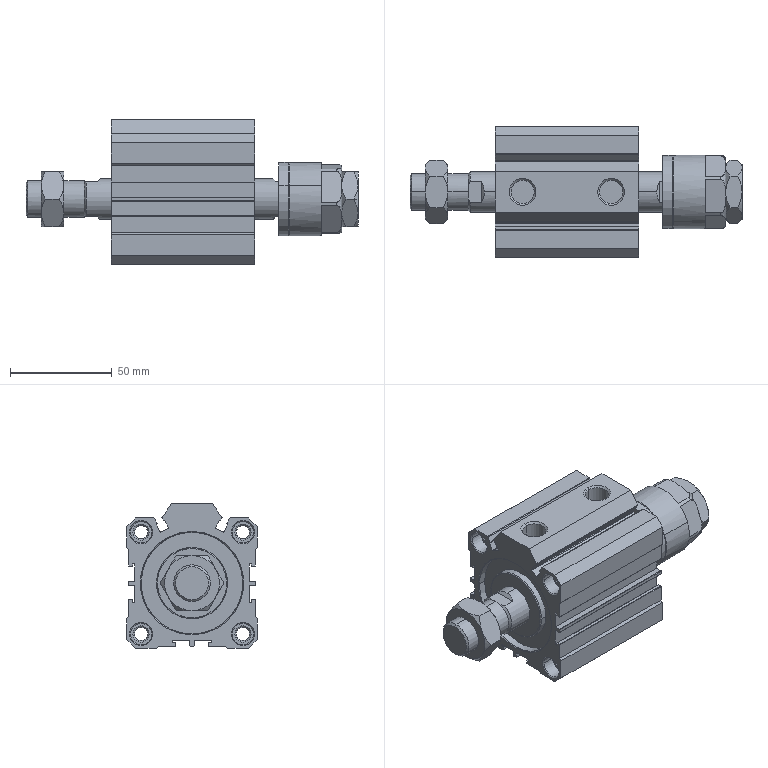Part | SolidWorks | features CompositeCurve 1 | 5 solids | 384 faces | box 163 x 64 x 71 mm | volume 272999 mm3 | plane 141 | cylinder 130 | cone 107 | spline 6 | commonest cylinder face diameters 0.4 x35 6.647 x16 10.5 x16 0.8 x15 6.5 x8 20 x8